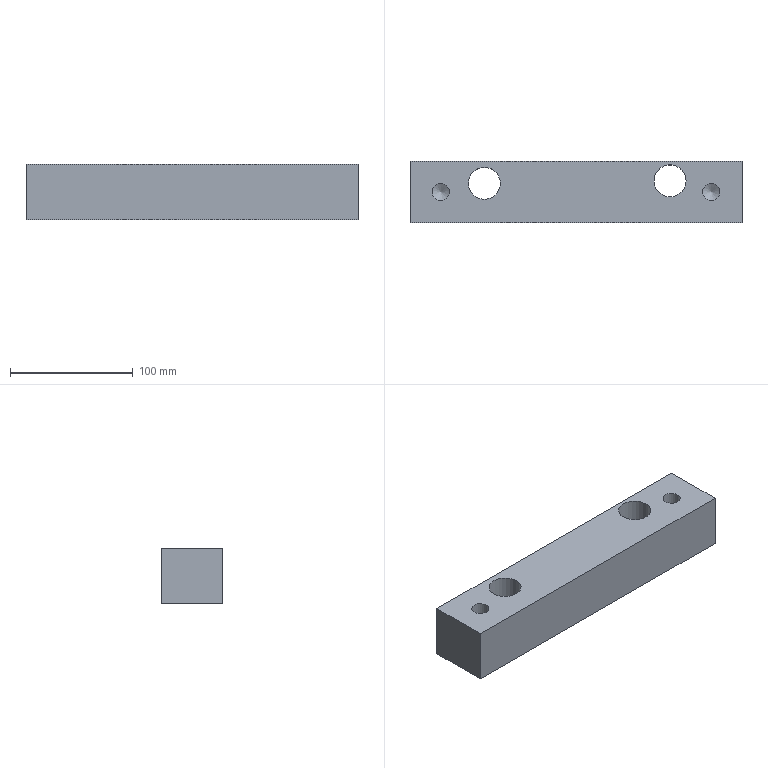Part | STEP file | 016_id2170_x_t | 1 solid | 12 faces | box 270 x 50 x 45 mm | volume 553311 mm3 | plane 6 | cylinder 4 | cone 2 | commonest cylinder face diameters 14 x2 26 x2
STEP:
#1=CARTESIAN_POINT('',(0.,0.,0.));
#2=DIRECTION('',(0.,0.,1.));
#3=DIRECTION('',(1.,0.,0.));
#4=AXIS2_PLACEMENT_3D('',#1,#2,#3);
#5=CARTESIAN_POINT('',(-131.5,16.,230.));
#6=VERTEX_POINT('',#5);
#7=CARTESIAN_POINT('',(-131.5,66.,230.));
#8=VERTEX_POINT('',#7);
#9=CARTESIAN_POINT('',(-131.5,66.,230.));
#10=DIRECTION('',(0.,1.,0.));
#11=VECTOR('',#10,1.);
#12=LINE('',#9,#11);
#13=CARTESIAN_POINT('',(303.5,-139.,230.));
#14=DIRECTION('',(0.,0.,1.));
#15=DIRECTION('',(0.,-1.,0.));
#16=AXIS2_PLACEMENT_3D('',#13,#14,#15);
#17=PLANE('',#16);
#18=CARTESIAN_POINT('',(-205.,-435.));
#19=DIRECTION('',(-1.,0.));
#20=VECTOR('',#19,1.);
#21=LINE('',#18,#20);
#22=(GEOMETRIC_REPRESENTATION_CONTEXT(2)PARAMETRIC_REPRESENTATION_CONTEXT()REPRESENTATION_CONTEXT('',''));
#23=DEFINITIONAL_REPRESENTATION('',(#21),#22);
#24=PCURVE('',#17,#23);
#25=CARTESIAN_POINT('',(-131.5,66.,428.5));
#26=DIRECTION('',(-1.,0.,0.));
#27=DIRECTION('',(0.,0.,1.));
#28=AXIS2_PLACEMENT_3D('',#25,#26,#27);
#29=PLANE('',#28);
#30=CARTESIAN_POINT('',(-198.5,0.));
#31=DIRECTION('',(0.,1.));
#32=VECTOR('',#31,1.);
#33=LINE('',#30,#32);
#34=(GEOMETRIC_REPRESENTATION_CONTEXT(2)PARAMETRIC_REPRESENTATION_CONTEXT()REPRESENTATION_CONTEXT('',''));
#35=DEFINITIONAL_REPRESENTATION('',(#33),#34);
#36=PCURVE('',#29,#35);
#37=SURFACE_CURVE('',#12,(#24,#36),.PCURVE_S1.);
#38=EDGE_CURVE('',#6,#8,#37,.T.);
#39=ORIENTED_EDGE('',*,*,#38,.F.);
#40=CARTESIAN_POINT('',(138.5,16.,230.));
#41=VERTEX_POINT('',#40);
#42=CARTESIAN_POINT('',(513.5,16.,230.));
#43=DIRECTION('',(-1.,0.,0.));
#44=VECTOR('',#43,1.);
#45=LINE('',#42,#44);
#46=CARTESIAN_POINT('',(-155.,210.));
#47=DIRECTION('',(0.,-1.));
#48=VECTOR('',#47,1.);
#49=LINE('',#46,#48);
#50=(GEOMETRIC_REPRESENTATION_CONTEXT(2)PARAMETRIC_REPRESENTATION_CONTEXT()REPRESENTATION_CONTEXT('',''));
#51=DEFINITIONAL_REPRESENTATION('',(#49),#50);
#52=PCURVE('',#17,#51);
#53=CARTESIAN_POINT('',(513.5,16.,428.5));
#54=DIRECTION('',(0.,1.,0.));
#55=DIRECTION('',(0.,0.,-1.));
#56=AXIS2_PLACEMENT_3D('',#53,#54,#55);
#57=PLANE('',#56);
#58=CARTESIAN_POINT('',(198.5,0.));
#59=DIRECTION('',(0.,1.));
#60=VECTOR('',#59,1.);
#61=LINE('',#58,#60);
#62=(GEOMETRIC_REPRESENTATION_CONTEXT(2)PARAMETRIC_REPRESENTATION_CONTEXT()REPRESENTATION_CONTEXT('',''));
#63=DEFINITIONAL_REPRESENTATION('',(#61),#62);
#64=PCURVE('',#57,#63);
#65=SURFACE_CURVE('',#45,(#52,#64),.PCURVE_S1.);
#66=EDGE_CURVE('',#41,#6,#65,.T.);
#67=ORIENTED_EDGE('',*,*,#66,.F.);
#68=CARTESIAN_POINT('',(138.5,66.,230.));
#69=VERTEX_POINT('',#68);
#70=CARTESIAN_POINT('',(138.5,66.,230.));
#71=DIRECTION('',(0.,1.,0.));
#72=VECTOR('',#71,1.);
#73=LINE('',#70,#72);
#74=CARTESIAN_POINT('',(-205.,-165.));
#75=DIRECTION('',(-1.,0.));
#76=VECTOR('',#75,1.);
#77=LINE('',#74,#76);
#78=(GEOMETRIC_REPRESENTATION_CONTEXT(2)PARAMETRIC_REPRESENTATION_CONTEXT()REPRESENTATION_CONTEXT('',''));
#79=DEFINITIONAL_REPRESENTATION('',(#77),#78);
#80=PCURVE('',#17,#79);
#81=CARTESIAN_POINT('',(138.5,66.,428.5));
#82=DIRECTION('',(-1.,0.,0.));
#83=DIRECTION('',(0.,0.,1.));
#84=AXIS2_PLACEMENT_3D('',#81,#82,#83);
#85=PLANE('',#84);
#86=CARTESIAN_POINT('',(-198.5,0.));
#87=DIRECTION('',(0.,1.));
#88=VECTOR('',#87,1.);
#89=LINE('',#86,#88);
#90=(GEOMETRIC_REPRESENTATION_CONTEXT(2)PARAMETRIC_REPRESENTATION_CONTEXT()REPRESENTATION_CONTEXT('',''));
#91=DEFINITIONAL_REPRESENTATION('',(#89),#90);
#92=PCURVE('',#85,#91);
#93=SURFACE_CURVE('',#73,(#80,#92),.PCURVE_S1.);
#94=EDGE_CURVE('',#41,#69,#93,.T.);
#95=ORIENTED_EDGE('',*,*,#94,.T.);
#96=CARTESIAN_POINT('',(513.5,66.,230.));
#97=DIRECTION('',(1.,0.,0.));
#98=VECTOR('',#97,1.);
#99=LINE('',#96,#98);
#100=CARTESIAN_POINT('',(-205.,210.));
#101=DIRECTION('',(0.,1.));
#102=VECTOR('',#101,1.);
#103=LINE('',#100,#102);
#104=(GEOMETRIC_REPRESENTATION_CONTEXT(2)PARAMETRIC_REPRESENTATION_CONTEXT()REPRESENTATION_CONTEXT('',''));
#105=DEFINITIONAL_REPRESENTATION('',(#103),#104);
#106=PCURVE('',#17,#105);
#107=CARTESIAN_POINT('',(513.5,66.,428.5));
#108=DIRECTION('',(0.,1.,0.));
#109=DIRECTION('',(0.,0.,-1.));
#110=AXIS2_PLACEMENT_3D('',#107,#108,#109);
#111=PLANE('',#110);
#112=CARTESIAN_POINT('',(198.5,0.));
#113=DIRECTION('',(0.,-1.));
#114=VECTOR('',#113,1.);
#115=LINE('',#112,#114);
#116=(GEOMETRIC_REPRESENTATION_CONTEXT(2)PARAMETRIC_REPRESENTATION_CONTEXT()REPRESENTATION_CONTEXT('',''));
#117=DEFINITIONAL_REPRESENTATION('',(#115),#116);
#118=PCURVE('',#111,#117);
#119=SURFACE_CURVE('',#99,(#106,#118),.PCURVE_S1.);
#120=EDGE_CURVE('',#8,#69,#119,.T.);
#121=ORIENTED_EDGE('',*,*,#120,.F.);
#122=EDGE_LOOP('',(#39,#67,#95,#121));
#123=FACE_BOUND('',#122,.T.);
#124=CARTESIAN_POINT('',(113.5,48.,230.));
#125=VERTEX_POINT('',#124);
#126=CARTESIAN_POINT('',(113.5,34.,230.));
#127=VERTEX_POINT('',#126);
#128=CARTESIAN_POINT('',(113.5,41.,230.));
#129=DIRECTION('',(0.,0.,1.));
#130=DIRECTION('',(0.,1.,0.));
#131=AXIS2_PLACEMENT_3D('',#128,#129,#130);
#132=CIRCLE('',#131,7.);
#133=CARTESIAN_POINT('',(-180.,-190.));
#134=DIRECTION('',(-1.,0.));
#135=AXIS2_PLACEMENT_2D('',#133,#134);
#136=CIRCLE('',#135,7.);
#137=(GEOMETRIC_REPRESENTATION_CONTEXT(2)PARAMETRIC_REPRESENTATION_CONTEXT()REPRESENTATION_CONTEXT('',''));
#138=DEFINITIONAL_REPRESENTATION('',(#136),#137);
#139=PCURVE('',#17,#138);
#140=CARTESIAN_POINT('',(113.5,41.,279.));
#141=DIRECTION('',(0.,0.,-1.));
#142=DIRECTION('',(0.,-1.,0.));
#143=AXIS2_PLACEMENT_3D('',#140,#141,#142);
#144=CYLINDRICAL_SURFACE('',#143,7.);
#145=CARTESIAN_POINT('',(3.142,49.));
#146=DIRECTION('',(-1.,0.));
#147=VECTOR('',#146,1.);
#148=LINE('',#145,#147);
#149=(GEOMETRIC_REPRESENTATION_CONTEXT(2)PARAMETRIC_REPRESENTATION_CONTEXT()REPRESENTATION_CONTEXT('',''));
#150=DEFINITIONAL_REPRESENTATION('',(#148),#149);
#151=PCURVE('',#144,#150);
#152=SURFACE_CURVE('',#132,(#139,#151),.PCURVE_S1.);
#153=EDGE_CURVE('',#125,#127,#152,.T.);
#154=ORIENTED_EDGE('',*,*,#153,.F.);
#155=CARTESIAN_POINT('',(113.5,41.,230.));
#156=DIRECTION('',(0.,0.,1.));
#157=DIRECTION('',(0.,1.,0.));
#158=AXIS2_PLACEMENT_3D('',#155,#156,#157);
#159=CIRCLE('',#158,7.);
#160=CARTESIAN_POINT('',(-180.,-190.));
#161=DIRECTION('',(-1.,0.));
#162=AXIS2_PLACEMENT_2D('',#160,#161);
#163=CIRCLE('',#162,7.);
#164=(GEOMETRIC_REPRESENTATION_CONTEXT(2)PARAMETRIC_REPRESENTATION_CONTEXT()REPRESENTATION_CONTEXT('',''));
#165=DEFINITIONAL_REPRESENTATION('',(#163),#164);
#166=PCURVE('',#17,#165);
#167=CARTESIAN_POINT('',(9.425,49.));
#168=DIRECTION('',(-1.,0.));
#169=VECTOR('',#168,1.);
#170=LINE('',#167,#169);
#171=(GEOMETRIC_REPRESENTATION_CONTEXT(2)PARAMETRIC_REPRESENTATION_CONTEXT()REPRESENTATION_CONTEXT('',''));
#172=DEFINITIONAL_REPRESENTATION('',(#170),#171);
#173=PCURVE('',#144,#172);
#174=SURFACE_CURVE('',#159,(#166,#173),.PCURVE_S1.);
#175=EDGE_CURVE('',#127,#125,#174,.T.);
#176=ORIENTED_EDGE('',*,*,#175,.F.);
#177=EDGE_LOOP('',(#154,#176));
#178=FACE_BOUND('',#177,.T.);
#179=CARTESIAN_POINT('',(-106.5,48.,230.));
#180=VERTEX_POINT('',#179);
#181=CARTESIAN_POINT('',(-106.5,34.,230.));
#182=VERTEX_POINT('',#181);
#183=CARTESIAN_POINT('',(-106.5,41.,230.));
#184=DIRECTION('',(0.,0.,-1.));
#185=DIRECTION('',(0.,1.,0.));
#186=AXIS2_PLACEMENT_3D('',#183,#184,#185);
#187=CIRCLE('',#186,7.);
#188=CARTESIAN_POINT('',(-187.,-410.));
#189=CARTESIAN_POINT('',(-187.,-397.876));
#190=CARTESIAN_POINT('',(-176.5,-403.938));
#191=CARTESIAN_POINT('',(-166.,-410.));
#192=CARTESIAN_POINT('',(-176.5,-416.062));
#193=CARTESIAN_POINT('',(-187.,-422.124));
#194=CARTESIAN_POINT('',(-187.,-410.));
#195=(BOUNDED_CURVE()B_SPLINE_CURVE(2,(#188,#189,#190,#191,#192,#193,#194),.UNSPECIFIED.,.T.,.F.)B_SPLINE_CURVE_WITH_KNOTS((1,2,2,2,2,1),(-2.094,0.,2.094,4.189,6.283,8.378),.UNSPECIFIED.)CURVE()GEOMETRIC_REPRESENTATION_ITEM()RATIONAL_B_SPLINE_CURVE((1.,0.5,1.,0.5,1.,0.5,1.))REPRESENTATION_ITEM(''));
#196=(GEOMETRIC_REPRESENTATION_CONTEXT(2)PARAMETRIC_REPRESENTATION_CONTEXT()REPRESENTATION_CONTEXT('',''));
#197=DEFINITIONAL_REPRESENTATION('',(#195),#196);
#198=PCURVE('',#17,#197);
#199=CARTESIAN_POINT('',(-106.5,41.,279.));
#200=DIRECTION('',(0.,0.,-1.));
#201=DIRECTION('',(0.,-1.,0.));
#202=AXIS2_PLACEMENT_3D('',#199,#200,#201);
#203=CYLINDRICAL_SURFACE('',#202,7.);
#204=CARTESIAN_POINT('',(3.142,49.));
#205=DIRECTION('',(1.,0.));
#206=VECTOR('',#205,1.);
#207=LINE('',#204,#206);
#208=(GEOMETRIC_REPRESENTATION_CONTEXT(2)PARAMETRIC_REPRESENTATION_CONTEXT()REPRESENTATION_CONTEXT('',''));
#209=DEFINITIONAL_REPRESENTATION('',(#207),#208);
#210=PCURVE('',#203,#209);
#211=SURFACE_CURVE('',#187,(#198,#210),.PCURVE_S1.);
#212=EDGE_CURVE('',#180,#182,#211,.T.);
#213=ORIENTED_EDGE('',*,*,#212,.T.);
#214=CARTESIAN_POINT('',(-106.5,41.,230.));
#215=DIRECTION('',(0.,0.,-1.));
#216=DIRECTION('',(0.,1.,0.));
#217=AXIS2_PLACEMENT_3D('',#214,#215,#216);
#218=CIRCLE('',#217,7.);
#219=CARTESIAN_POINT('',(-187.,-410.));
#220=CARTESIAN_POINT('',(-187.,-397.876));
#221=CARTESIAN_POINT('',(-176.5,-403.938));
#222=CARTESIAN_POINT('',(-166.,-410.));
#223=CARTESIAN_POINT('',(-176.5,-416.062));
#224=CARTESIAN_POINT('',(-187.,-422.124));
#225=CARTESIAN_POINT('',(-187.,-410.));
#226=(BOUNDED_CURVE()B_SPLINE_CURVE(2,(#219,#220,#221,#222,#223,#224,#225),.UNSPECIFIED.,.T.,.F.)B_SPLINE_CURVE_WITH_KNOTS((1,2,2,2,2,1),(-2.094,0.,2.094,4.189,6.283,8.378),.UNSPECIFIED.)CURVE()GEOMETRIC_REPRESENTATION_ITEM()RATIONAL_B_SPLINE_CURVE((1.,0.5,1.,0.5,1.,0.5,1.))REPRESENTATION_ITEM(''));
#227=(GEOMETRIC_REPRESENTATION_CONTEXT(2)PARAMETRIC_REPRESENTATION_CONTEXT()REPRESENTATION_CONTEXT('',''));
#228=DEFINITIONAL_REPRESENTATION('',(#226),#227);
#229=PCURVE('',#17,#228);
#230=CARTESIAN_POINT('',(-3.142,49.));
#231=DIRECTION('',(1.,0.));
#232=VECTOR('',#231,1.);
#233=LINE('',#230,#232);
#234=(GEOMETRIC_REPRESENTATION_CONTEXT(2)PARAMETRIC_REPRESENTATION_CONTEXT()REPRESENTATION_CONTEXT('',''));
#235=DEFINITIONAL_REPRESENTATION('',(#233),#234);
#236=PCURVE('',#203,#235);
#237=SURFACE_CURVE('',#218,(#229,#236),.PCURVE_S1.);
#238=EDGE_CURVE('',#182,#180,#237,.T.);
#239=ORIENTED_EDGE('',*,*,#238,.T.);
#240=EDGE_LOOP('',(#213,#239));
#241=FACE_BOUND('',#240,.T.);
#242=CARTESIAN_POINT('',(-58.02,48.053,230.));
#243=VERTEX_POINT('',#242);
#244=CARTESIAN_POINT('',(-71.02,48.053,230.));
#245=DIRECTION('',(0.,0.,1.));
#246=DIRECTION('',(1.,0.,0.));
#247=AXIS2_PLACEMENT_3D('',#244,#245,#246);
#248=CIRCLE('',#247,13.);
#249=CARTESIAN_POINT('',(-187.053,-374.52));
#250=DIRECTION('',(0.,1.));
#251=AXIS2_PLACEMENT_2D('',#249,#250);
#252=CIRCLE('',#251,13.);
#253=(GEOMETRIC_REPRESENTATION_CONTEXT(2)PARAMETRIC_REPRESENTATION_CONTEXT()REPRESENTATION_CONTEXT('',''));
#254=DEFINITIONAL_REPRESENTATION('',(#252),#253);
#255=PCURVE('',#17,#254);
#256=CARTESIAN_POINT('',(-71.02,48.053,360.));
#257=DIRECTION('',(0.,0.,-1.));
#258=DIRECTION('',(-1.,0.,0.));
#259=AXIS2_PLACEMENT_3D('',#256,#257,#258);
#260=CYLINDRICAL_SURFACE('',#259,13.);
#261=CARTESIAN_POINT('',(9.425,130.));
#262=DIRECTION('',(-1.,0.));
#263=VECTOR('',#262,1.);
#264=LINE('',#261,#263);
#265=(GEOMETRIC_REPRESENTATION_CONTEXT(2)PARAMETRIC_REPRESENTATION_CONTEXT()REPRESENTATION_CONTEXT('',''));
#266=DEFINITIONAL_REPRESENTATION('',(#264),#265);
#267=PCURVE('',#260,#266);
#268=SURFACE_CURVE('',#248,(#255,#267),.PCURVE_S1.);
#269=EDGE_CURVE('',#243,#243,#268,.T.);
#270=ORIENTED_EDGE('',*,*,#269,.F.);
#271=EDGE_LOOP('',(#270));
#272=FACE_BOUND('',#271,.T.);
#273=CARTESIAN_POINT('',(92.98,50.053,230.));
#274=VERTEX_POINT('',#273);
#275=CARTESIAN_POINT('',(79.98,50.053,230.));
#276=DIRECTION('',(0.,0.,-1.));
#277=DIRECTION('',(1.,0.,0.));
#278=AXIS2_PLACEMENT_3D('',#275,#276,#277);
#279=CIRCLE('',#278,13.);
#280=CARTESIAN_POINT('',(-189.053,-210.52));
#281=CARTESIAN_POINT('',(-166.536,-210.52));
#282=CARTESIAN_POINT('',(-177.795,-230.02));
#283=CARTESIAN_POINT('',(-189.053,-249.52));
#284=CARTESIAN_POINT('',(-200.311,-230.02));
#285=CARTESIAN_POINT('',(-211.57,-210.52));
#286=CARTESIAN_POINT('',(-189.053,-210.52));
#287=(BOUNDED_CURVE()B_SPLINE_CURVE(2,(#280,#281,#282,#283,#284,#285,#286),.UNSPECIFIED.,.T.,.F.)B_SPLINE_CURVE_WITH_KNOTS((1,2,2,2,2,1),(-2.094,0.,2.094,4.189,6.283,8.378),.UNSPECIFIED.)CURVE()GEOMETRIC_REPRESENTATION_ITEM()RATIONAL_B_SPLINE_CURVE((1.,0.5,1.,0.5,1.,0.5,1.))REPRESENTATION_ITEM(''));
#288=(GEOMETRIC_REPRESENTATION_CONTEXT(2)PARAMETRIC_REPRESENTATION_CONTEXT()REPRESENTATION_CONTEXT('',''));
#289=DEFINITIONAL_REPRESENTATION('',(#287),#288);
#290=PCURVE('',#17,#289);
#291=CARTESIAN_POINT('',(79.98,50.053,360.));
#292=DIRECTION('',(0.,0.,-1.));
#293=DIRECTION('',(-1.,0.,0.));
#294=AXIS2_PLACEMENT_3D('',#291,#292,#293);
#295=CYLINDRICAL_SURFACE('',#294,13.);
#296=CARTESIAN_POINT('',(3.142,130.));
#297=DIRECTION('',(1.,0.));
#298=VECTOR('',#297,1.);
#299=LINE('',#296,#298);
#300=(GEOMETRIC_REPRESENTATION_CONTEXT(2)PARAMETRIC_REPRESENTATION_CONTEXT()REPRESENTATION_CONTEXT('',''));
#301=DEFINITIONAL_REPRESENTATION('',(#299),#300);
#302=PCURVE('',#295,#301);
#303=SURFACE_CURVE('',#279,(#290,#302),.PCURVE_S1.);
#304=EDGE_CURVE('',#274,#274,#303,.T.);
#305=ORIENTED_EDGE('',*,*,#304,.T.);
#306=EDGE_LOOP('',(#305));
#307=FACE_BOUND('',#306,.T.);
#308=ADVANCED_FACE('',(#123,#178,#241,#272,#307),#17,.T.);
#309=CARTESIAN_POINT('',(138.5,16.,185.));
#310=VERTEX_POINT('',#309);
#311=CARTESIAN_POINT('',(138.5,66.,185.));
#312=VERTEX_POINT('',#311);
#313=CARTESIAN_POINT('',(138.5,66.,185.));
#314=DIRECTION('',(0.,1.,0.));
#315=VECTOR('',#314,1.);
#316=LINE('',#313,#315);
#317=CARTESIAN_POINT('',(513.5,66.,185.));
#318=DIRECTION('',(0.,0.,1.));
#319=DIRECTION('',(1.,0.,0.));
#320=AXIS2_PLACEMENT_3D('',#317,#318,#319);
#321=PLANE('',#320);
#322=CARTESIAN_POINT('',(-375.,0.));
#323=DIRECTION('',(0.,1.));
#324=VECTOR('',#323,1.);
#325=LINE('',#322,#324);
#326=(GEOMETRIC_REPRESENTATION_CONTEXT(2)PARAMETRIC_REPRESENTATION_CONTEXT()REPRESENTATION_CONTEXT('',''));
#327=DEFINITIONAL_REPRESENTATION('',(#325),#326);
#328=PCURVE('',#321,#327);
#329=CARTESIAN_POINT('',(-243.5,0.));
#330=DIRECTION('',(0.,1.));
#331=VECTOR('',#330,1.);
#332=LINE('',#329,#331);
#333=(GEOMETRIC_REPRESENTATION_CONTEXT(2)PARAMETRIC_REPRESENTATION_CONTEXT()REPRESENTATION_CONTEXT('',''));
#334=DEFINITIONAL_REPRESENTATION('',(#332),#333);
#335=PCURVE('',#85,#334);
#336=SURFACE_CURVE('',#316,(#328,#335),.PCURVE_S1.);
#337=EDGE_CURVE('',#310,#312,#336,.T.);
#338=ORIENTED_EDGE('',*,*,#337,.F.);
#339=CARTESIAN_POINT('',(-131.5,16.,185.));
#340=VERTEX_POINT('',#339);
#341=CARTESIAN_POINT('',(513.5,16.,185.));
#342=DIRECTION('',(-1.,0.,0.));
#343=VECTOR('',#342,1.);
#344=LINE('',#341,#343);
#345=CARTESIAN_POINT('',(0.,-50.));
#346=DIRECTION('',(-1.,0.));
#347=VECTOR('',#346,1.);
#348=LINE('',#345,#347);
#349=(GEOMETRIC_REPRESENTATION_CONTEXT(2)PARAMETRIC_REPRESENTATION_CONTEXT()REPRESENTATION_CONTEXT('',''));
#350=DEFINITIONAL_REPRESENTATION('',(#348),#349);
#351=PCURVE('',#321,#350);
#352=CARTESIAN_POINT('',(243.5,0.));
#353=DIRECTION('',(0.,1.));
#354=VECTOR('',#353,1.);
#355=LINE('',#352,#354);
#356=(GEOMETRIC_REPRESENTATION_CONTEXT(2)PARAMETRIC_REPRESENTATION_CONTEXT()REPRESENTATION_CONTEXT('',''));
#357=DEFINITIONAL_REPRESENTATION('',(#355),#356);
#358=PCURVE('',#57,#357);
#359=SURFACE_CURVE('',#344,(#351,#358),.PCURVE_S1.);
#360=EDGE_CURVE('',#310,#340,#359,.T.);
#361=ORIENTED_EDGE('',*,*,#360,.T.);
#362=CARTESIAN_POINT('',(-131.5,66.,185.));
#363=VERTEX_POINT('',#362);
#364=CARTESIAN_POINT('',(-131.5,66.,185.));
#365=DIRECTION('',(0.,1.,0.));
#366=VECTOR('',#365,1.);
#367=LINE('',#364,#366);
#368=CARTESIAN_POINT('',(-645.,0.));
#369=DIRECTION('',(0.,1.));
#370=VECTOR('',#369,1.);
#371=LINE('',#368,#370);
#372=(GEOMETRIC_REPRESENTATION_CONTEXT(2)PARAMETRIC_REPRESENTATION_CONTEXT()REPRESENTATION_CONTEXT('',''));
#373=DEFINITIONAL_REPRESENTATION('',(#371),#372);
#374=PCURVE('',#321,#373);
#375=CARTESIAN_POINT('',(-243.5,0.));
#376=DIRECTION('',(0.,1.));
#377=VECTOR('',#376,1.);
#378=LINE('',#375,#377);
#379=(GEOMETRIC_REPRESENTATION_CONTEXT(2)PARAMETRIC_REPRESENTATION_CONTEXT()REPRESENTATION_CONTEXT('',''));
#380=DEFINITIONAL_REPRESENTATION('',(#378),#379);
#381=PCURVE('',#29,#380);
#382=SURFACE_CURVE('',#367,(#374,#381),.PCURVE_S1.);
#383=EDGE_CURVE('',#340,#363,#382,.T.);
#384=ORIENTED_EDGE('',*,*,#383,.T.);
#385=CARTESIAN_POINT('',(513.5,66.,185.));
#386=DIRECTION('',(-1.,0.,0.));
#387=VECTOR('',#386,1.);
#388=LINE('',#385,#387);
#389=CARTESIAN_POINT('',(0.,0.));
#390=DIRECTION('',(-1.,0.));
#391=VECTOR('',#390,1.);
#392=LINE('',#389,#391);
#393=(GEOMETRIC_REPRESENTATION_CONTEXT(2)PARAMETRIC_REPRESENTATION_CONTEXT()REPRESENTATION_CONTEXT('',''));
#394=DEFINITIONAL_REPRESENTATION('',(#392),#393);
#395=PCURVE('',#321,#394);
#396=CARTESIAN_POINT('',(243.5,0.));
#397=DIRECTION('',(0.,1.));
#398=VECTOR('',#397,1.);
#399=LINE('',#396,#398);
#400=(GEOMETRIC_REPRESENTATION_CONTEXT(2)PARAMETRIC_REPRESENTATION_CONTEXT()REPRESENTATION_CONTEXT('',''));
#401=DEFINITIONAL_REPRESENTATION('',(#399),#400);
#402=PCURVE('',#111,#401);
#403=SURFACE_CURVE('',#388,(#395,#402),.PCURVE_S1.);
#404=EDGE_CURVE('',#312,#363,#403,.T.);
#405=ORIENTED_EDGE('',*,*,#404,.F.);
#406=EDGE_LOOP('',(#338,#361,#384,#405));
#407=FACE_BOUND('',#406,.T.);
#408=CARTESIAN_POINT('',(-58.02,48.053,185.));
#409=VERTEX_POINT('',#408);
#410=CARTESIAN_POINT('',(-71.02,48.053,185.));
#411=DIRECTION('',(0.,0.,1.));
#412=DIRECTION('',(1.,0.,0.));
#413=AXIS2_PLACEMENT_3D('',#410,#411,#412);
#414=CIRCLE('',#413,13.);
#415=CARTESIAN_POINT('',(-584.52,-17.947));
#416=DIRECTION('',(1.,0.));
#417=AXIS2_PLACEMENT_2D('',#415,#416);
#418=CIRCLE('',#417,13.);
#419=(GEOMETRIC_REPRESENTATION_CONTEXT(2)PARAMETRIC_REPRESENTATION_CONTEXT()REPRESENTATION_CONTEXT('',''));
#420=DEFINITIONAL_REPRESENTATION('',(#418),#419);
#421=PCURVE('',#321,#420);
#422=CARTESIAN_POINT('',(9.425,175.));
#423=DIRECTION('',(-1.,0.));
#424=VECTOR('',#423,1.);
#425=LINE('',#422,#424);
#426=(GEOMETRIC_REPRESENTATION_CONTEXT(2)PARAMETRIC_REPRESENTATION_CONTEXT()REPRESENTATION_CONTEXT('',''));
#427=DEFINITIONAL_REPRESENTATION('',(#425),#426);
#428=PCURVE('',#260,#427);
#429=SURFACE_CURVE('',#414,(#421,#428),.PCURVE_S1.);
#430=EDGE_CURVE('',#409,#409,#429,.T.);
#431=ORIENTED_EDGE('',*,*,#430,.T.);
#432=EDGE_LOOP('',(#431));
#433=FACE_BOUND('',#432,.T.);
#434=CARTESIAN_POINT('',(92.98,50.053,185.));
#435=VERTEX_POINT('',#434);
#436=CARTESIAN_POINT('',(79.98,50.053,185.));
#437=DIRECTION('',(0.,0.,-1.));
#438=DIRECTION('',(1.,0.,0.));
#439=AXIS2_PLACEMENT_3D('',#436,#437,#438);
#440=CIRCLE('',#439,13.);
#441=CARTESIAN_POINT('',(-420.52,-15.947));
#442=CARTESIAN_POINT('',(-420.52,-38.464));
#443=CARTESIAN_POINT('',(-440.02,-27.205));
#444=CARTESIAN_POINT('',(-459.52,-15.947));
#445=CARTESIAN_POINT('',(-440.02,-4.689));
#446=CARTESIAN_POINT('',(-420.52,6.57));
#447=CARTESIAN_POINT('',(-420.52,-15.947));
#448=(BOUNDED_CURVE()B_SPLINE_CURVE(2,(#441,#442,#443,#444,#445,#446,#447),.UNSPECIFIED.,.T.,.F.)B_SPLINE_CURVE_WITH_KNOTS((1,2,2,2,2,1),(-2.094,0.,2.094,4.189,6.283,8.378),.UNSPECIFIED.)CURVE()GEOMETRIC_REPRESENTATION_ITEM()RATIONAL_B_SPLINE_CURVE((1.,0.5,1.,0.5,1.,0.5,1.))REPRESENTATION_ITEM(''));
#449=(GEOMETRIC_REPRESENTATION_CONTEXT(2)PARAMETRIC_REPRESENTATION_CONTEXT()REPRESENTATION_CONTEXT('',''));
#450=DEFINITIONAL_REPRESENTATION('',(#448),#449);
#451=PCURVE('',#321,#450);
#452=CARTESIAN_POINT('',(3.142,175.));
#453=DIRECTION('',(1.,0.));
#454=VECTOR('',#453,1.);
#455=LINE('',#452,#454);
#456=(GEOMETRIC_REPRESENTATION_CONTEXT(2)PARAMETRIC_REPRESENTATION_CONTEXT()REPRESENTATION_CONTEXT('',''));
#457=DEFINITIONAL_REPRESENTATION('',(#455),#456);
#458=PCURVE('',#295,#457);
#459=SURFACE_CURVE('',#440,(#451,#458),.PCURVE_S1.);
#460=EDGE_CURVE('',#435,#435,#459,.T.);
#461=ORIENTED_EDGE('',*,*,#460,.F.);
#462=EDGE_LOOP('',(#461));
#463=FACE_BOUND('',#462,.T.);
#464=ADVANCED_FACE('',(#407,#433,#463),#321,.F.);
#465=ORIENTED_EDGE('',*,*,#66,.T.);
#466=CARTESIAN_POINT('',(-131.5,16.,428.5));
#467=DIRECTION('',(0.,0.,1.));
#468=VECTOR('',#467,1.);
#469=LINE('',#466,#468);
#470=CARTESIAN_POINT('',(0.,645.));
#471=DIRECTION('',(-1.,0.));
#472=VECTOR('',#471,1.);
#473=LINE('',#470,#472);
#474=(GEOMETRIC_REPRESENTATION_CONTEXT(2)PARAMETRIC_REPRESENTATION_CONTEXT()REPRESENTATION_CONTEXT('',''));
#475=DEFINITIONAL_REPRESENTATION('',(#473),#474);
#476=PCURVE('',#57,#475);
#477=CARTESIAN_POINT('',(0.,-50.));
#478=DIRECTION('',(1.,0.));
#479=VECTOR('',#478,1.);
#480=LINE('',#477,#479);
#481=(GEOMETRIC_REPRESENTATION_CONTEXT(2)PARAMETRIC_REPRESENTATION_CONTEXT()REPRESENTATION_CONTEXT('',''));
#482=DEFINITIONAL_REPRESENTATION('',(#480),#481);
#483=PCURVE('',#29,#482);
#484=SURFACE_CURVE('',#469,(#476,#483),.PCURVE_S1.);
#485=EDGE_CURVE('',#340,#6,#484,.T.);
#486=ORIENTED_EDGE('',*,*,#485,.F.);
#487=ORIENTED_EDGE('',*,*,#360,.F.);
#488=CARTESIAN_POINT('',(138.5,16.,428.5));
#489=DIRECTION('',(0.,0.,-1.));
#490=VECTOR('',#489,1.);
#491=LINE('',#488,#490);
#492=CARTESIAN_POINT('',(0.,375.));
#493=DIRECTION('',(1.,0.));
#494=VECTOR('',#493,1.);
#495=LINE('',#492,#494);
#496=(GEOMETRIC_REPRESENTATION_CONTEXT(2)PARAMETRIC_REPRESENTATION_CONTEXT()REPRESENTATION_CONTEXT('',''));
#497=DEFINITIONAL_REPRESENTATION('',(#495),#496);
#498=PCURVE('',#57,#497);
#499=CARTESIAN_POINT('',(0.,-50.));
#500=DIRECTION('',(-1.,0.));
#501=VECTOR('',#500,1.);
#502=LINE('',#499,#501);
#503=(GEOMETRIC_REPRESENTATION_CONTEXT(2)PARAMETRIC_REPRESENTATION_CONTEXT()REPRESENTATION_CONTEXT('',''));
#504=DEFINITIONAL_REPRESENTATION('',(#502),#503);
#505=PCURVE('',#85,#504);
#506=SURFACE_CURVE('',#491,(#498,#505),.PCURVE_S1.);
#507=EDGE_CURVE('',#41,#310,#506,.T.);
#508=ORIENTED_EDGE('',*,*,#507,.F.);
#509=EDGE_LOOP('',(#465,#486,#487,#508));
#510=FACE_BOUND('',#509,.T.);
#511=ADVANCED_FACE('',(#510),#57,.F.);
#512=ORIENTED_EDGE('',*,*,#94,.F.);
#513=ORIENTED_EDGE('',*,*,#507,.T.);
#514=ORIENTED_EDGE('',*,*,#337,.T.);
#515=CARTESIAN_POINT('',(138.5,66.,428.5));
#516=DIRECTION('',(0.,0.,-1.));
#517=VECTOR('',#516,1.);
#518=LINE('',#515,#517);
#519=CARTESIAN_POINT('',(0.,0.));
#520=DIRECTION('',(-1.,0.));
#521=VECTOR('',#520,1.);
#522=LINE('',#519,#521);
#523=(GEOMETRIC_REPRESENTATION_CONTEXT(2)PARAMETRIC_REPRESENTATION_CONTEXT()REPRESENTATION_CONTEXT('',''));
#524=DEFINITIONAL_REPRESENTATION('',(#522),#523);
#525=PCURVE('',#85,#524);
#526=CARTESIAN_POINT('',(0.,375.));
#527=DIRECTION('',(1.,0.));
#528=VECTOR('',#527,1.);
#529=LINE('',#526,#528);
#530=(GEOMETRIC_REPRESENTATION_CONTEXT(2)PARAMETRIC_REPRESENTATION_CONTEXT()REPRESENTATION_CONTEXT('',''));
#531=DEFINITIONAL_REPRESENTATION('',(#529),#530);
#532=PCURVE('',#111,#531);
#533=SURFACE_CURVE('',#518,(#525,#532),.PCURVE_S1.);
#534=EDGE_CURVE('',#69,#312,#533,.T.);
#535=ORIENTED_EDGE('',*,*,#534,.F.);
#536=EDGE_LOOP('',(#512,#513,#514,#535));
#537=FACE_BOUND('',#536,.T.);
#538=ADVANCED_FACE('',(#537),#85,.F.);
#539=CARTESIAN_POINT('',(-131.5,66.,428.5));
#540=DIRECTION('',(0.,0.,1.));
#541=VECTOR('',#540,1.);
#542=LINE('',#539,#541);
#543=CARTESIAN_POINT('',(0.,645.));
#544=DIRECTION('',(-1.,0.));
#545=VECTOR('',#544,1.);
#546=LINE('',#543,#545);
#547=(GEOMETRIC_REPRESENTATION_CONTEXT(2)PARAMETRIC_REPRESENTATION_CONTEXT()REPRESENTATION_CONTEXT('',''));
#548=DEFINITIONAL_REPRESENTATION('',(#546),#547);
#549=PCURVE('',#111,#548);
#550=CARTESIAN_POINT('',(0.,0.));
#551=DIRECTION('',(1.,0.));
#552=VECTOR('',#551,1.);
#553=LINE('',#550,#552);
#554=(GEOMETRIC_REPRESENTATION_CONTEXT(2)PARAMETRIC_REPRESENTATION_CONTEXT()REPRESENTATION_CONTEXT('',''));
#555=DEFINITIONAL_REPRESENTATION('',(#553),#554);
#556=PCURVE('',#29,#555);
#557=SURFACE_CURVE('',#542,(#549,#556),.PCURVE_S1.);
#558=EDGE_CURVE('',#363,#8,#557,.T.);
#559=ORIENTED_EDGE('',*,*,#558,.T.);
#560=ORIENTED_EDGE('',*,*,#120,.T.);
#561=ORIENTED_EDGE('',*,*,#534,.T.);
#562=ORIENTED_EDGE('',*,*,#404,.T.);
#563=EDGE_LOOP('',(#559,#560,#561,#562));
#564=FACE_BOUND('',#563,.T.);
#565=ADVANCED_FACE('',(#564),#111,.T.);
#566=ORIENTED_EDGE('',*,*,#485,.T.);
#567=ORIENTED_EDGE('',*,*,#38,.T.);
#568=ORIENTED_EDGE('',*,*,#558,.F.);
#569=ORIENTED_EDGE('',*,*,#383,.F.);
#570=EDGE_LOOP('',(#566,#567,#568,#569));
#571=FACE_BOUND('',#570,.T.);
#572=ADVANCED_FACE('',(#571),#29,.T.);
#573=ORIENTED_EDGE('',*,*,#212,.T.);
#574=CARTESIAN_POINT('',(-106.5,34.,210.541));
#575=VERTEX_POINT('',#574);
#576=CARTESIAN_POINT('',(-106.5,34.,230.));
#577=CARTESIAN_POINT('',(-106.5,34.,210.541));
#578=B_SPLINE_CURVE_WITH_KNOTS('',1,(#576,#577),.UNSPECIFIED.,.F.,.F.,(2,2),(49.,68.459),.PIECEWISE_BEZIER_KNOTS.);
#579=CARTESIAN_POINT('',(6.283,0.));
#580=DIRECTION('',(0.,1.));
#581=VECTOR('',#580,1.);
#582=LINE('',#579,#581);
#583=(GEOMETRIC_REPRESENTATION_CONTEXT(2)PARAMETRIC_REPRESENTATION_CONTEXT()REPRESENTATION_CONTEXT('',''));
#584=DEFINITIONAL_REPRESENTATION('',(#582),#583);
#585=PCURVE('',#203,#584);
#586=CARTESIAN_POINT('',(0.,0.));
#587=DIRECTION('',(0.,1.));
#588=VECTOR('',#587,1.);
#589=LINE('',#586,#588);
#590=(GEOMETRIC_REPRESENTATION_CONTEXT(2)PARAMETRIC_REPRESENTATION_CONTEXT()REPRESENTATION_CONTEXT('',''));
#591=DEFINITIONAL_REPRESENTATION('',(#589),#590);
#592=PCURVE('',#203,#591);
#593=SEAM_CURVE('',#578,(#585,#592),.PCURVE_S1.);
#594=EDGE_CURVE('',#182,#575,#593,.T.);
#595=ORIENTED_EDGE('',*,*,#594,.T.);
#596=CARTESIAN_POINT('',(-106.5,48.,210.541));
#597=VERTEX_POINT('',#596);
#598=CARTESIAN_POINT('',(-106.5,41.,210.541));
#599=DIRECTION('',(0.,0.,-1.));
#600=DIRECTION('',(0.,-1.,0.));
#601=AXIS2_PLACEMENT_3D('',#598,#599,#600);
#602=CIRCLE('',#601,7.);
#603=CARTESIAN_POINT('',(0.,68.459));
#604=DIRECTION('',(1.,0.));
#605=VECTOR('',#604,1.);
#606=LINE('',#603,#605);
#607=(GEOMETRIC_REPRESENTATION_CONTEXT(2)PARAMETRIC_REPRESENTATION_CONTEXT()REPRESENTATION_CONTEXT('',''));
#608=DEFINITIONAL_REPRESENTATION('',(#606),#607);
#609=PCURVE('',#203,#608);
#610=CARTESIAN_POINT('',(-106.5,41.,210.541));
#611=DIRECTION('',(0.,0.,1.));
#612=DIRECTION('',(0.,1.,0.));
#613=AXIS2_PLACEMENT_3D('',#610,#611,#612);
#614=CONICAL_SURFACE('',#613,7.,1.047);
#615=CARTESIAN_POINT('',(9.425,0.));
#616=DIRECTION('',(-1.,0.));
#617=VECTOR('',#616,1.);
#618=LINE('',#615,#617);
#619=(GEOMETRIC_REPRESENTATION_CONTEXT(2)PARAMETRIC_REPRESENTATION_CONTEXT()REPRESENTATION_CONTEXT('',''));
#620=DEFINITIONAL_REPRESENTATION('',(#618),#619);
#621=PCURVE('',#614,#620);
#622=SURFACE_CURVE('',#602,(#609,#621),.PCURVE_S1.);
#623=EDGE_CURVE('',#597,#575,#622,.T.);
#624=ORIENTED_EDGE('',*,*,#623,.F.);
#625=CARTESIAN_POINT('',(-106.5,41.,210.541));
#626=DIRECTION('',(0.,0.,-1.));
#627=DIRECTION('',(0.,-1.,0.));
#628=AXIS2_PLACEMENT_3D('',#625,#626,#627);
#629=CIRCLE('',#628,7.);
#630=CARTESIAN_POINT('',(0.,68.459));
#631=DIRECTION('',(1.,0.));
#632=VECTOR('',#631,1.);
#633=LINE('',#630,#632);
#634=(GEOMETRIC_REPRESENTATION_CONTEXT(2)PARAMETRIC_REPRESENTATION_CONTEXT()REPRESENTATION_CONTEXT('',''));
#635=DEFINITIONAL_REPRESENTATION('',(#633),#634);
#636=PCURVE('',#203,#635);
#637=CARTESIAN_POINT('',(3.142,0.));
#638=DIRECTION('',(-1.,0.));
#639=VECTOR('',#638,1.);
#640=LINE('',#637,#639);
#641=(GEOMETRIC_REPRESENTATION_CONTEXT(2)PARAMETRIC_REPRESENTATION_CONTEXT()REPRESENTATION_CONTEXT('',''));
#642=DEFINITIONAL_REPRESENTATION('',(#640),#641);
#643=PCURVE('',#614,#642);
#644=SURFACE_CURVE('',#629,(#636,#643),.PCURVE_S1.);
#645=EDGE_CURVE('',#575,#597,#644,.T.);
#646=ORIENTED_EDGE('',*,*,#645,.F.);
#647=ORIENTED_EDGE('',*,*,#594,.F.);
#648=ORIENTED_EDGE('',*,*,#238,.T.);
#649=EDGE_LOOP('',(#573,#595,#624,#646,#647,#648));
#650=FACE_BOUND('',#649,.F.);
#651=ADVANCED_FACE('',(#650),#203,.F.);
#652=CARTESIAN_POINT('',(-106.5,41.,206.5));
#653=VERTEX_POINT('',#652);
#654=CARTESIAN_POINT('',(-106.5,41.,206.5));
#655=CARTESIAN_POINT('',(-106.5,48.,210.541));
#656=B_SPLINE_CURVE_WITH_KNOTS('',1,(#654,#655),.UNSPECIFIED.,.F.,.F.,(2,2),(-8.083,0.),.PIECEWISE_BEZIER_KNOTS.);
#657=CARTESIAN_POINT('',(6.283,0.));
#658=DIRECTION('',(0.,1.));
#659=VECTOR('',#658,1.);
#660=LINE('',#657,#659);
#661=(GEOMETRIC_REPRESENTATION_CONTEXT(2)PARAMETRIC_REPRESENTATION_CONTEXT()REPRESENTATION_CONTEXT('',''));
#662=DEFINITIONAL_REPRESENTATION('',(#660),#661);
#663=PCURVE('',#614,#662);
#664=CARTESIAN_POINT('',(0.,0.));
#665=DIRECTION('',(0.,1.));
#666=VECTOR('',#665,1.);
#667=LINE('',#664,#666);
#668=(GEOMETRIC_REPRESENTATION_CONTEXT(2)PARAMETRIC_REPRESENTATION_CONTEXT()REPRESENTATION_CONTEXT('',''));
#669=DEFINITIONAL_REPRESENTATION('',(#667),#668);
#670=PCURVE('',#614,#669);
#671=SEAM_CURVE('',#656,(#663,#670),.PCURVE_S1.);
#672=EDGE_CURVE('',#653,#597,#671,.T.);
#673=ORIENTED_EDGE('',*,*,#672,.T.);
#674=ORIENTED_EDGE('',*,*,#623,.T.);
#675=ORIENTED_EDGE('',*,*,#645,.T.);
#676=ORIENTED_EDGE('',*,*,#672,.F.);
#677=EDGE_LOOP('',(#673,#674,#675,#676));
#678=FACE_BOUND('',#677,.F.);
#679=ADVANCED_FACE('',(#678),#614,.F.);
#680=ORIENTED_EDGE('',*,*,#175,.F.);
#681=CARTESIAN_POINT('',(113.5,34.,210.541));
#682=VERTEX_POINT('',#681);
#683=CARTESIAN_POINT('',(113.5,34.,230.));
#684=CARTESIAN_POINT('',(113.5,34.,210.541));
#685=B_SPLINE_CURVE_WITH_KNOTS('',1,(#683,#684),.UNSPECIFIED.,.F.,.F.,(2,2),(49.,68.459),.PIECEWISE_BEZIER_KNOTS.);
#686=CARTESIAN_POINT('',(6.283,0.));
#687=DIRECTION('',(0.,1.));
#688=VECTOR('',#687,1.);
#689=LINE('',#686,#688);
#690=(GEOMETRIC_REPRESENTATION_CONTEXT(2)PARAMETRIC_REPRESENTATION_CONTEXT()REPRESENTATION_CONTEXT('',''));
#691=DEFINITIONAL_REPRESENTATION('',(#689),#690);
#692=PCURVE('',#144,#691);
#693=CARTESIAN_POINT('',(0.,0.));
#694=DIRECTION('',(0.,1.));
#695=VECTOR('',#694,1.);
#696=LINE('',#693,#695);
#697=(GEOMETRIC_REPRESENTATION_CONTEXT(2)PARAMETRIC_REPRESENTATION_CONTEXT()REPRESENTATION_CONTEXT('',''));
#698=DEFINITIONAL_REPRESENTATION('',(#696),#697);
#699=PCURVE('',#144,#698);
#700=SEAM_CURVE('',#685,(#692,#699),.PCURVE_S1.);
#701=EDGE_CURVE('',#127,#682,#700,.T.);
#702=ORIENTED_EDGE('',*,*,#701,.T.);
#703=CARTESIAN_POINT('',(113.5,48.,210.541));
#704=VERTEX_POINT('',#703);
#705=CARTESIAN_POINT('',(113.5,41.,210.541));
#706=DIRECTION('',(0.,0.,1.));
#707=DIRECTION('',(0.,-1.,0.));
#708=AXIS2_PLACEMENT_3D('',#705,#706,#707);
#709=CIRCLE('',#708,7.);
#710=CARTESIAN_POINT('',(6.283,68.459));
#711=DIRECTION('',(-1.,0.));
#712=VECTOR('',#711,1.);
#713=LINE('',#710,#712);
#714=(GEOMETRIC_REPRESENTATION_CONTEXT(2)PARAMETRIC_REPRESENTATION_CONTEXT()REPRESENTATION_CONTEXT('',''));
#715=DEFINITIONAL_REPRESENTATION('',(#713),#714);
#716=PCURVE('',#144,#715);
#717=CARTESIAN_POINT('',(113.5,41.,210.541));
#718=DIRECTION('',(0.,0.,1.));
#719=DIRECTION('',(0.,1.,0.));
#720=AXIS2_PLACEMENT_3D('',#717,#718,#719);
#721=CONICAL_SURFACE('',#720,7.,1.047);
#722=CARTESIAN_POINT('',(3.142,0.));
#723=DIRECTION('',(1.,0.));
#724=VECTOR('',#723,1.);
#725=LINE('',#722,#724);
#726=(GEOMETRIC_REPRESENTATION_CONTEXT(2)PARAMETRIC_REPRESENTATION_CONTEXT()REPRESENTATION_CONTEXT('',''));
#727=DEFINITIONAL_REPRESENTATION('',(#725),#726);
#728=PCURVE('',#721,#727);
#729=SURFACE_CURVE('',#709,(#716,#728),.PCURVE_S1.);
#730=EDGE_CURVE('',#682,#704,#729,.T.);
#731=ORIENTED_EDGE('',*,*,#730,.T.);
#732=CARTESIAN_POINT('',(113.5,41.,210.541));
#733=DIRECTION('',(0.,0.,1.));
#734=DIRECTION('',(0.,-1.,0.));
#735=AXIS2_PLACEMENT_3D('',#732,#733,#734);
#736=CIRCLE('',#735,7.);
#737=CARTESIAN_POINT('',(6.283,68.459));
#738=DIRECTION('',(-1.,0.));
#739=VECTOR('',#738,1.);
#740=LINE('',#737,#739);
#741=(GEOMETRIC_REPRESENTATION_CONTEXT(2)PARAMETRIC_REPRESENTATION_CONTEXT()REPRESENTATION_CONTEXT('',''));
#742=DEFINITIONAL_REPRESENTATION('',(#740),#741);
#743=PCURVE('',#144,#742);
#744=CARTESIAN_POINT('',(-3.142,0.));
#745=DIRECTION('',(1.,0.));
#746=VECTOR('',#745,1.);
#747=LINE('',#744,#746);
#748=(GEOMETRIC_REPRESENTATION_CONTEXT(2)PARAMETRIC_REPRESENTATION_CONTEXT()REPRESENTATION_CONTEXT('',''));
#749=DEFINITIONAL_REPRESENTATION('',(#747),#748);
#750=PCURVE('',#721,#749);
#751=SURFACE_CURVE('',#736,(#743,#750),.PCURVE_S1.);
#752=EDGE_CURVE('',#704,#682,#751,.T.);
#753=ORIENTED_EDGE('',*,*,#752,.T.);
#754=ORIENTED_EDGE('',*,*,#701,.F.);
#755=ORIENTED_EDGE('',*,*,#153,.F.);
#756=EDGE_LOOP('',(#680,#702,#731,#753,#754,#755));
#757=FACE_BOUND('',#756,.F.);
#758=ADVANCED_FACE('',(#757),#144,.F.);
#759=CARTESIAN_POINT('',(113.5,41.,206.5));
#760=VERTEX_POINT('',#759);
#761=CARTESIAN_POINT('',(113.5,41.,206.5));
#762=CARTESIAN_POINT('',(113.5,48.,210.541));
#763=B_SPLINE_CURVE_WITH_KNOTS('',1,(#761,#762),.UNSPECIFIED.,.F.,.F.,(2,2),(-8.083,0.),.PIECEWISE_BEZIER_KNOTS.);
#764=CARTESIAN_POINT('',(6.283,0.));
#765=DIRECTION('',(0.,1.));
#766=VECTOR('',#765,1.);
#767=LINE('',#764,#766);
#768=(GEOMETRIC_REPRESENTATION_CONTEXT(2)PARAMETRIC_REPRESENTATION_CONTEXT()REPRESENTATION_CONTEXT('',''));
#769=DEFINITIONAL_REPRESENTATION('',(#767),#768);
#770=PCURVE('',#721,#769);
#771=CARTESIAN_POINT('',(0.,0.));
#772=DIRECTION('',(0.,1.));
#773=VECTOR('',#772,1.);
#774=LINE('',#771,#773);
#775=(GEOMETRIC_REPRESENTATION_CONTEXT(2)PARAMETRIC_REPRESENTATION_CONTEXT()REPRESENTATION_CONTEXT('',''));
#776=DEFINITIONAL_REPRESENTATION('',(#774),#775);
#777=PCURVE('',#721,#776);
#778=SEAM_CURVE('',#763,(#770,#777),.PCURVE_S1.);
#779=EDGE_CURVE('',#760,#704,#778,.T.);
#780=ORIENTED_EDGE('',*,*,#779,.T.);
#781=ORIENTED_EDGE('',*,*,#730,.F.);
#782=ORIENTED_EDGE('',*,*,#752,.F.);
#783=ORIENTED_EDGE('',*,*,#779,.F.);
#784=EDGE_LOOP('',(#780,#781,#782,#783));
#785=FACE_BOUND('',#784,.F.);
#786=ADVANCED_FACE('',(#785),#721,.F.);
#787=ORIENTED_EDGE('',*,*,#269,.F.);
#788=CARTESIAN_POINT('',(-58.02,48.053,230.));
#789=CARTESIAN_POINT('',(-58.02,48.053,185.));
#790=B_SPLINE_CURVE_WITH_KNOTS('',1,(#788,#789),.UNSPECIFIED.,.F.,.F.,(2,2),(130.,175.),.PIECEWISE_BEZIER_KNOTS.);
#791=CARTESIAN_POINT('',(9.425,0.));
#792=DIRECTION('',(0.,1.));
#793=VECTOR('',#792,1.);
#794=LINE('',#791,#793);
#795=(GEOMETRIC_REPRESENTATION_CONTEXT(2)PARAMETRIC_REPRESENTATION_CONTEXT()REPRESENTATION_CONTEXT('',''));
#796=DEFINITIONAL_REPRESENTATION('',(#794),#795);
#797=PCURVE('',#260,#796);
#798=CARTESIAN_POINT('',(3.142,0.));
#799=DIRECTION('',(0.,1.));
#800=VECTOR('',#799,1.);
#801=LINE('',#798,#800);
#802=(GEOMETRIC_REPRESENTATION_CONTEXT(2)PARAMETRIC_REPRESENTATION_CONTEXT()REPRESENTATION_CONTEXT('',''));
#803=DEFINITIONAL_REPRESENTATION('',(#801),#802);
#804=PCURVE('',#260,#803);
#805=SEAM_CURVE('',#790,(#797,#804),.PCURVE_S1.);
#806=EDGE_CURVE('',#243,#409,#805,.T.);
#807=ORIENTED_EDGE('',*,*,#806,.T.);
#808=ORIENTED_EDGE('',*,*,#430,.T.);
#809=ORIENTED_EDGE('',*,*,#806,.F.);
#810=EDGE_LOOP('',(#787,#807,#808,#809));
#811=FACE_BOUND('',#810,.F.);
#812=ADVANCED_FACE('',(#811),#260,.F.);
#813=ORIENTED_EDGE('',*,*,#304,.T.);
#814=CARTESIAN_POINT('',(92.98,50.053,230.));
#815=CARTESIAN_POINT('',(92.98,50.053,185.));
#816=B_SPLINE_CURVE_WITH_KNOTS('',1,(#814,#815),.UNSPECIFIED.,.F.,.F.,(2,2),(130.,175.),.PIECEWISE_BEZIER_KNOTS.);
#817=CARTESIAN_POINT('',(9.425,0.));
#818=DIRECTION('',(0.,1.));
#819=VECTOR('',#818,1.);
#820=LINE('',#817,#819);
#821=(GEOMETRIC_REPRESENTATION_CONTEXT(2)PARAMETRIC_REPRESENTATION_CONTEXT()REPRESENTATION_CONTEXT('',''));
#822=DEFINITIONAL_REPRESENTATION('',(#820),#821);
#823=PCURVE('',#295,#822);
#824=CARTESIAN_POINT('',(3.142,0.));
#825=DIRECTION('',(0.,1.));
#826=VECTOR('',#825,1.);
#827=LINE('',#824,#826);
#828=(GEOMETRIC_REPRESENTATION_CONTEXT(2)PARAMETRIC_REPRESENTATION_CONTEXT()REPRESENTATION_CONTEXT('',''));
#829=DEFINITIONAL_REPRESENTATION('',(#827),#828);
#830=PCURVE('',#295,#829);
#831=SEAM_CURVE('',#816,(#823,#830),.PCURVE_S1.);
#832=EDGE_CURVE('',#274,#435,#831,.T.);
#833=ORIENTED_EDGE('',*,*,#832,.T.);
#834=ORIENTED_EDGE('',*,*,#460,.F.);
#835=ORIENTED_EDGE('',*,*,#832,.F.);
#836=EDGE_LOOP('',(#813,#833,#834,#835));
#837=FACE_BOUND('',#836,.F.);
#838=ADVANCED_FACE('',(#837),#295,.F.);
#839=CLOSED_SHELL('',(#308,#464,#511,#538,#565,#572,#651,#679,#758,#786,#812,#838));
#840=MANIFOLD_SOLID_BREP('',#839);
#841=(LENGTH_UNIT()NAMED_UNIT(*)SI_UNIT(.MILLI.,.METRE.));
#842=UNCERTAINTY_MEASURE_WITH_UNIT(LENGTH_MEASURE(0.000005),#841,'','');
#843=(NAMED_UNIT(*)PLANE_ANGLE_UNIT()SI_UNIT($,.RADIAN.));
#844=(NAMED_UNIT(*)SI_UNIT($,.STERADIAN.)SOLID_ANGLE_UNIT());
#845=(GEOMETRIC_REPRESENTATION_CONTEXT(3)GLOBAL_UNCERTAINTY_ASSIGNED_CONTEXT((#842))GLOBAL_UNIT_ASSIGNED_CONTEXT((#841,#843,#844))REPRESENTATION_CONTEXT('',''));
#846=ADVANCED_BREP_SHAPE_REPRESENTATION('',(#4,#840),#845);